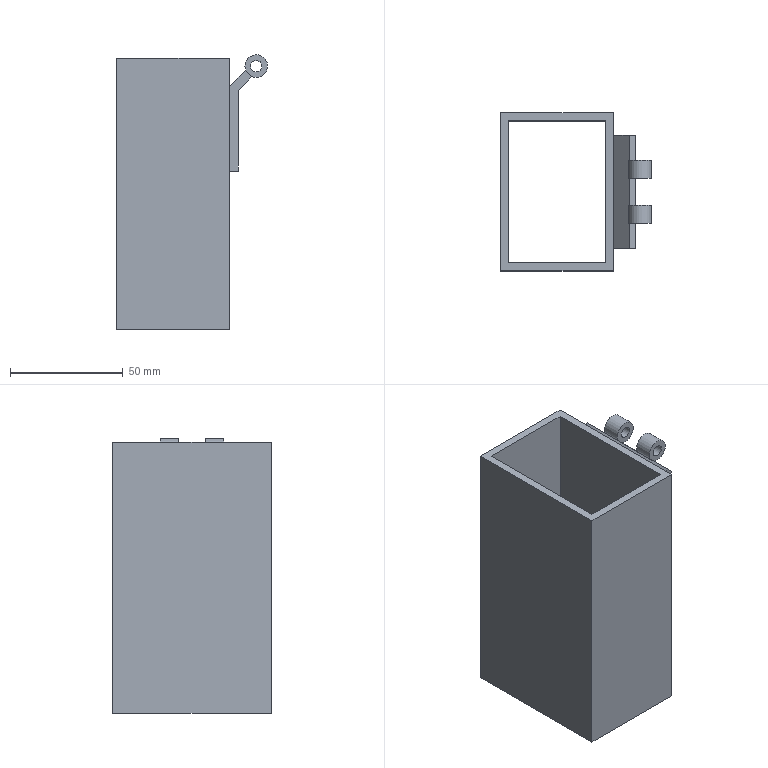Part | NX | features solid 2 | 1 solid | 25 faces | box 66.879 x 70 x 121.464 mm | volume 105008 mm3 | plane 21 | cylinder 4 | commonest cylinder face diameters 5 x2 10 x2
STEP:
#1=CARTESIAN_POINT('',(-1609.757,505.,4.586));
#2=VERTEX_POINT('',#1);
#3=CARTESIAN_POINT('',(-1609.757,455.,4.586));
#4=VERTEX_POINT('',#3);
#5=CARTESIAN_POINT('',(-1609.757,505.,4.586));
#6=DIRECTION('',(0.,1.,0.));
#7=VECTOR('',#6,1000.);
#8=LINE('',#5,#7);
#9=EDGE_CURVE('',#2,#4,#8,.F.);
#10=ORIENTED_EDGE('',*,*,#9,.T.);
#11=CARTESIAN_POINT('',(-1609.757,455.,-31.172));
#12=VERTEX_POINT('',#11);
#13=CARTESIAN_POINT('',(-1609.757,455.,18.828));
#14=DIRECTION('',(0.,0.,1.));
#15=VECTOR('',#14,1000.);
#16=LINE('',#13,#15);
#17=EDGE_CURVE('',#4,#12,#16,.F.);
#18=ORIENTED_EDGE('',*,*,#17,.T.);
#19=CARTESIAN_POINT('',(-1609.757,505.,-31.172));
#20=VERTEX_POINT('',#19);
#21=CARTESIAN_POINT('',(-1609.757,505.,-31.172));
#22=DIRECTION('',(0.,-1.,0.));
#23=VECTOR('',#22,1000.);
#24=LINE('',#21,#23);
#25=EDGE_CURVE('',#20,#12,#24,.T.);
#26=ORIENTED_EDGE('',*,*,#25,.F.);
#27=CARTESIAN_POINT('',(-1609.757,505.,18.828));
#28=DIRECTION('',(0.,0.,1.));
#29=VECTOR('',#28,1000.);
#30=LINE('',#27,#29);
#31=EDGE_CURVE('',#2,#20,#30,.F.);
#32=ORIENTED_EDGE('',*,*,#31,.F.);
#33=EDGE_LOOP('',(#10,#18,#26,#32));
#34=FACE_BOUND('',#33,.T.);
#35=CARTESIAN_POINT('',(-1609.757,505.,18.828));
#36=DIRECTION('',(1.,0.,0.));
#37=DIRECTION('',(0.,-1.,0.));
#38=AXIS2_PLACEMENT_3D('',#35,#36,#37);
#39=PLANE('',#38);
#40=ADVANCED_FACE('',(#34),#39,.T.);
#41=CARTESIAN_POINT('',(-1606.687,455.,13.313));
#42=VERTEX_POINT('',#41);
#43=CARTESIAN_POINT('',(-1613.757,455.,6.243));
#44=VERTEX_POINT('',#43);
#45=CARTESIAN_POINT('',(-1605.464,455.,14.536));
#46=DIRECTION('',(0.7071,0.,0.7071));
#47=VECTOR('',#46,1000.);
#48=LINE('',#45,#47);
#49=EDGE_CURVE('',#42,#44,#48,.F.);
#50=ORIENTED_EDGE('',*,*,#49,.T.);
#51=CARTESIAN_POINT('',(-1613.757,455.,-31.172));
#52=VERTEX_POINT('',#51);
#53=CARTESIAN_POINT('',(-1613.757,455.,18.828));
#54=DIRECTION('',(0.,0.,1.));
#55=VECTOR('',#54,1000.);
#56=LINE('',#53,#55);
#57=EDGE_CURVE('',#44,#52,#56,.F.);
#58=ORIENTED_EDGE('',*,*,#57,.T.);
#59=CARTESIAN_POINT('',(-1609.757,455.,-31.172));
#60=DIRECTION('',(-1.,0.,0.));
#61=VECTOR('',#60,1000.);
#62=LINE('',#59,#61);
#63=EDGE_CURVE('',#12,#52,#62,.T.);
#64=ORIENTED_EDGE('',*,*,#63,.F.);
#65=ORIENTED_EDGE('',*,*,#17,.F.);
#66=CARTESIAN_POINT('',(-1603.859,455.,10.485));
#67=VERTEX_POINT('',#66);
#68=CARTESIAN_POINT('',(-1614.707,455.,-0.364));
#69=DIRECTION('',(-0.7071,0.,-0.7071));
#70=VECTOR('',#69,1000.);
#71=LINE('',#68,#70);
#72=EDGE_CURVE('',#4,#67,#71,.F.);
#73=ORIENTED_EDGE('',*,*,#72,.T.);
#74=CARTESIAN_POINT('',(-1608.808,455.,15.434));
#75=DIRECTION('',(-0.7071,0.,0.7071));
#76=VECTOR('',#75,1000.);
#77=LINE('',#74,#76);
#78=EDGE_CURVE('',#42,#67,#77,.F.);
#79=ORIENTED_EDGE('',*,*,#78,.F.);
#80=EDGE_LOOP('',(#50,#58,#64,#65,#73,#79));
#81=FACE_BOUND('',#80,.T.);
#82=CARTESIAN_POINT('',(-1609.757,455.,18.828));
#83=DIRECTION('',(0.,-1.,0.));
#84=DIRECTION('',(-1.,0.,0.));
#85=AXIS2_PLACEMENT_3D('',#82,#83,#84);
#86=PLANE('',#85);
#87=ADVANCED_FACE('',(#81),#86,.T.);
#88=CARTESIAN_POINT('',(-1606.687,505.,13.313));
#89=VERTEX_POINT('',#88);
#90=CARTESIAN_POINT('',(-1613.757,505.,6.243));
#91=VERTEX_POINT('',#90);
#92=CARTESIAN_POINT('',(-1617.536,505.,2.464));
#93=DIRECTION('',(-0.7071,0.,-0.7071));
#94=VECTOR('',#93,1000.);
#95=LINE('',#92,#94);
#96=EDGE_CURVE('',#89,#91,#95,.T.);
#97=ORIENTED_EDGE('',*,*,#96,.F.);
#98=CARTESIAN_POINT('',(-1603.859,505.,10.485));
#99=VERTEX_POINT('',#98);
#100=CARTESIAN_POINT('',(-1608.808,505.,15.434));
#101=DIRECTION('',(-0.7071,0.,0.7071));
#102=VECTOR('',#101,1000.);
#103=LINE('',#100,#102);
#104=EDGE_CURVE('',#99,#89,#103,.T.);
#105=ORIENTED_EDGE('',*,*,#104,.F.);
#106=CARTESIAN_POINT('',(-1614.707,505.,-0.364));
#107=DIRECTION('',(0.7071,0.,0.7071));
#108=VECTOR('',#107,1000.);
#109=LINE('',#106,#108);
#110=EDGE_CURVE('',#2,#99,#109,.T.);
#111=ORIENTED_EDGE('',*,*,#110,.F.);
#112=ORIENTED_EDGE('',*,*,#31,.T.);
#113=CARTESIAN_POINT('',(-1613.757,505.,-31.172));
#114=VERTEX_POINT('',#113);
#115=CARTESIAN_POINT('',(-1609.757,505.,-31.172));
#116=DIRECTION('',(-1.,0.,0.));
#117=VECTOR('',#116,1000.);
#118=LINE('',#115,#117);
#119=EDGE_CURVE('',#20,#114,#118,.T.);
#120=ORIENTED_EDGE('',*,*,#119,.T.);
#121=CARTESIAN_POINT('',(-1613.757,505.,18.828));
#122=DIRECTION('',(0.,0.,1.));
#123=VECTOR('',#122,1000.);
#124=LINE('',#121,#123);
#125=EDGE_CURVE('',#91,#114,#124,.F.);
#126=ORIENTED_EDGE('',*,*,#125,.F.);
#127=EDGE_LOOP('',(#97,#105,#111,#112,#120,#126));
#128=FACE_BOUND('',#127,.T.);
#129=CARTESIAN_POINT('',(-1609.757,505.,18.828));
#130=DIRECTION('',(0.,-1.,0.));
#131=DIRECTION('',(-1.,0.,0.));
#132=AXIS2_PLACEMENT_3D('',#129,#130,#131);
#133=PLANE('',#132);
#134=ADVANCED_FACE('',(#128),#133,.F.);
#135=CARTESIAN_POINT('',(-1613.757,505.,-31.172));
#136=DIRECTION('',(0.,-1.,0.));
#137=VECTOR('',#136,1000.);
#138=LINE('',#135,#137);
#139=EDGE_CURVE('',#114,#52,#138,.T.);
#140=ORIENTED_EDGE('',*,*,#139,.F.);
#141=ORIENTED_EDGE('',*,*,#119,.F.);
#142=ORIENTED_EDGE('',*,*,#25,.T.);
#143=ORIENTED_EDGE('',*,*,#63,.T.);
#144=EDGE_LOOP('',(#140,#141,#142,#143));
#145=FACE_BOUND('',#144,.T.);
#146=CARTESIAN_POINT('',(-1609.757,505.,-31.172));
#147=DIRECTION('',(0.,0.,1.));
#148=DIRECTION('',(0.,-1.,0.));
#149=AXIS2_PLACEMENT_3D('',#146,#147,#148);
#150=PLANE('',#149);
#151=ADVANCED_FACE('',(#145),#150,.F.);
#152=CARTESIAN_POINT('',(-1613.757,505.,6.243));
#153=DIRECTION('',(0.,-1.,0.));
#154=VECTOR('',#153,1000.);
#155=LINE('',#152,#154);
#156=EDGE_CURVE('',#91,#44,#155,.T.);
#157=ORIENTED_EDGE('',*,*,#156,.T.);
#158=ORIENTED_EDGE('',*,*,#49,.F.);
#159=CARTESIAN_POINT('',(-1606.687,505.,13.313));
#160=DIRECTION('',(0.,1.,0.));
#161=VECTOR('',#160,1000.);
#162=LINE('',#159,#161);
#163=EDGE_CURVE('',#89,#42,#162,.F.);
#164=ORIENTED_EDGE('',*,*,#163,.F.);
#165=ORIENTED_EDGE('',*,*,#96,.T.);
#166=EDGE_LOOP('',(#157,#158,#164,#165));
#167=FACE_BOUND('',#166,.T.);
#168=CARTESIAN_POINT('',(-1617.536,505.,2.464));
#169=DIRECTION('',(-0.7071,0.,0.7071));
#170=DIRECTION('',(0.,-1.,0.));
#171=AXIS2_PLACEMENT_3D('',#168,#169,#170);
#172=PLANE('',#171);
#173=ADVANCED_FACE('',(#167),#172,.T.);
#174=ORIENTED_EDGE('',*,*,#72,.F.);
#175=ORIENTED_EDGE('',*,*,#9,.F.);
#176=ORIENTED_EDGE('',*,*,#110,.T.);
#177=CARTESIAN_POINT('',(-1603.859,505.,10.485));
#178=DIRECTION('',(0.,1.,0.));
#179=VECTOR('',#178,1000.);
#180=LINE('',#177,#179);
#181=EDGE_CURVE('',#67,#99,#180,.T.);
#182=ORIENTED_EDGE('',*,*,#181,.F.);
#183=EDGE_LOOP('',(#174,#175,#176,#182));
#184=FACE_BOUND('',#183,.T.);
#185=CARTESIAN_POINT('',(-1614.707,505.,-0.364));
#186=DIRECTION('',(-0.7071,0.,0.7071));
#187=DIRECTION('',(0.,-1.,0.));
#188=AXIS2_PLACEMENT_3D('',#185,#186,#187);
#189=PLANE('',#188);
#190=ADVANCED_FACE('',(#184),#189,.F.);
#191=CARTESIAN_POINT('',(-1606.263,466.,12.889));
#192=VERTEX_POINT('',#191);
#193=CARTESIAN_POINT('',(-1606.263,474.,12.889));
#194=VERTEX_POINT('',#193);
#195=CARTESIAN_POINT('',(-1606.263,455.,12.889));
#196=DIRECTION('',(0.,1.,0.));
#197=VECTOR('',#196,1000.);
#198=LINE('',#195,#197);
#199=EDGE_CURVE('',#192,#194,#198,.T.);
#200=ORIENTED_EDGE('',*,*,#199,.T.);
#201=CARTESIAN_POINT('',(-1604.283,474.,10.909));
#202=VERTEX_POINT('',#201);
#203=CARTESIAN_POINT('',(-1608.808,474.,15.434));
#204=DIRECTION('',(0.7071,0.,-0.7071));
#205=VECTOR('',#204,1000.);
#206=LINE('',#203,#205);
#207=EDGE_CURVE('',#194,#202,#206,.T.);
#208=ORIENTED_EDGE('',*,*,#207,.T.);
#209=CARTESIAN_POINT('',(-1604.283,466.,10.909));
#210=VERTEX_POINT('',#209);
#211=CARTESIAN_POINT('',(-1604.283,455.,10.909));
#212=DIRECTION('',(0.,1.,0.));
#213=VECTOR('',#212,1000.);
#214=LINE('',#211,#213);
#215=EDGE_CURVE('',#202,#210,#214,.F.);
#216=ORIENTED_EDGE('',*,*,#215,.T.);
#217=CARTESIAN_POINT('',(-1608.808,466.,15.434));
#218=DIRECTION('',(0.7071,0.,-0.7071));
#219=VECTOR('',#218,1000.);
#220=LINE('',#217,#219);
#221=EDGE_CURVE('',#192,#210,#220,.T.);
#222=ORIENTED_EDGE('',*,*,#221,.F.);
#223=EDGE_LOOP('',(#200,#208,#216,#222));
#224=FACE_BOUND('',#223,.T.);
#225=CARTESIAN_POINT('',(-1606.263,486.,12.889));
#226=VERTEX_POINT('',#225);
#227=CARTESIAN_POINT('',(-1606.263,494.,12.889));
#228=VERTEX_POINT('',#227);
#229=CARTESIAN_POINT('',(-1606.263,475.,12.889));
#230=DIRECTION('',(0.,1.,0.));
#231=VECTOR('',#230,1000.);
#232=LINE('',#229,#231);
#233=EDGE_CURVE('',#226,#228,#232,.T.);
#234=ORIENTED_EDGE('',*,*,#233,.T.);
#235=CARTESIAN_POINT('',(-1604.283,494.,10.909));
#236=VERTEX_POINT('',#235);
#237=CARTESIAN_POINT('',(-1608.808,494.,15.434));
#238=DIRECTION('',(0.7071,0.,-0.7071));
#239=VECTOR('',#238,1000.);
#240=LINE('',#237,#239);
#241=EDGE_CURVE('',#228,#236,#240,.T.);
#242=ORIENTED_EDGE('',*,*,#241,.T.);
#243=CARTESIAN_POINT('',(-1604.283,486.,10.909));
#244=VERTEX_POINT('',#243);
#245=CARTESIAN_POINT('',(-1604.283,475.,10.909));
#246=DIRECTION('',(0.,1.,0.));
#247=VECTOR('',#246,1000.);
#248=LINE('',#245,#247);
#249=EDGE_CURVE('',#236,#244,#248,.F.);
#250=ORIENTED_EDGE('',*,*,#249,.T.);
#251=CARTESIAN_POINT('',(-1608.808,486.,15.434));
#252=DIRECTION('',(0.7071,0.,-0.7071));
#253=VECTOR('',#252,1000.);
#254=LINE('',#251,#253);
#255=EDGE_CURVE('',#226,#244,#254,.T.);
#256=ORIENTED_EDGE('',*,*,#255,.F.);
#257=EDGE_LOOP('',(#234,#242,#250,#256));
#258=FACE_BOUND('',#257,.T.);
#259=ORIENTED_EDGE('',*,*,#163,.T.);
#260=ORIENTED_EDGE('',*,*,#78,.T.);
#261=ORIENTED_EDGE('',*,*,#181,.T.);
#262=ORIENTED_EDGE('',*,*,#104,.T.);
#263=EDGE_LOOP('',(#259,#260,#261,#262));
#264=FACE_BOUND('',#263,.T.);
#265=CARTESIAN_POINT('',(-1608.808,505.,15.434));
#266=DIRECTION('',(-0.7071,0.,-0.7071));
#267=DIRECTION('',(0.7071,0.,-0.7071));
#268=AXIS2_PLACEMENT_3D('',#265,#266,#267);
#269=PLANE('',#268);
#270=ADVANCED_FACE('',(#224,#258,#264),#269,.F.);
#271=CARTESIAN_POINT('',(-1613.757,515.,-101.172));
#272=VERTEX_POINT('',#271);
#273=CARTESIAN_POINT('',(-1613.757,445.,-101.172));
#274=VERTEX_POINT('',#273);
#275=CARTESIAN_POINT('',(-1613.757,530.,-101.172));
#276=DIRECTION('',(0.,1.,0.));
#277=VECTOR('',#276,1000.);
#278=LINE('',#275,#277);
#279=EDGE_CURVE('',#272,#274,#278,.F.);
#280=ORIENTED_EDGE('',*,*,#279,.F.);
#281=CARTESIAN_POINT('',(-1613.757,515.,18.828));
#282=VERTEX_POINT('',#281);
#283=CARTESIAN_POINT('',(-1613.757,515.,18.828));
#284=DIRECTION('',(0.,0.,1.));
#285=VECTOR('',#284,1000.);
#286=LINE('',#283,#285);
#287=EDGE_CURVE('',#282,#272,#286,.F.);
#288=ORIENTED_EDGE('',*,*,#287,.F.);
#289=CARTESIAN_POINT('',(-1613.757,445.,18.828));
#290=VERTEX_POINT('',#289);
#291=CARTESIAN_POINT('',(-1613.757,530.,18.828));
#292=DIRECTION('',(0.,-1.,0.));
#293=VECTOR('',#292,1000.);
#294=LINE('',#291,#293);
#295=EDGE_CURVE('',#282,#290,#294,.T.);
#296=ORIENTED_EDGE('',*,*,#295,.T.);
#297=CARTESIAN_POINT('',(-1613.757,445.,18.828));
#298=DIRECTION('',(0.,0.,-1.));
#299=VECTOR('',#298,1000.);
#300=LINE('',#297,#299);
#301=EDGE_CURVE('',#290,#274,#300,.T.);
#302=ORIENTED_EDGE('',*,*,#301,.T.);
#303=EDGE_LOOP('',(#280,#288,#296,#302));
#304=FACE_BOUND('',#303,.T.);
#305=ORIENTED_EDGE('',*,*,#57,.F.);
#306=ORIENTED_EDGE('',*,*,#156,.F.);
#307=ORIENTED_EDGE('',*,*,#125,.T.);
#308=ORIENTED_EDGE('',*,*,#139,.T.);
#309=EDGE_LOOP('',(#305,#306,#307,#308));
#310=FACE_BOUND('',#309,.T.);
#311=CARTESIAN_POINT('',(-1613.757,530.,18.828));
#312=DIRECTION('',(1.,0.,0.));
#313=DIRECTION('',(0.,-1.,0.));
#314=AXIS2_PLACEMENT_3D('',#311,#312,#313);
#315=PLANE('',#314);
#316=ADVANCED_FACE('',(#304,#310),#315,.T.);
#317=ORIENTED_EDGE('',*,*,#301,.F.);
#318=CARTESIAN_POINT('',(-1663.757,445.,18.828));
#319=VERTEX_POINT('',#318);
#320=CARTESIAN_POINT('',(-1613.757,445.,18.828));
#321=DIRECTION('',(1.,0.,0.));
#322=VECTOR('',#321,1000.);
#323=LINE('',#320,#322);
#324=EDGE_CURVE('',#290,#319,#323,.F.);
#325=ORIENTED_EDGE('',*,*,#324,.T.);
#326=CARTESIAN_POINT('',(-1663.757,445.,-101.172));
#327=VERTEX_POINT('',#326);
#328=CARTESIAN_POINT('',(-1663.757,445.,18.828));
#329=DIRECTION('',(0.,0.,1.));
#330=VECTOR('',#329,1000.);
#331=LINE('',#328,#330);
#332=EDGE_CURVE('',#319,#327,#331,.F.);
#333=ORIENTED_EDGE('',*,*,#332,.T.);
#334=CARTESIAN_POINT('',(-1613.757,445.,-101.172));
#335=DIRECTION('',(1.,0.,0.));
#336=VECTOR('',#335,1000.);
#337=LINE('',#334,#336);
#338=EDGE_CURVE('',#274,#327,#337,.F.);
#339=ORIENTED_EDGE('',*,*,#338,.F.);
#340=EDGE_LOOP('',(#317,#325,#333,#339));
#341=FACE_BOUND('',#340,.T.);
#342=CARTESIAN_POINT('',(-1613.757,445.,18.828));
#343=DIRECTION('',(0.,-1.,0.));
#344=DIRECTION('',(-1.,0.,0.));
#345=AXIS2_PLACEMENT_3D('',#342,#343,#344);
#346=PLANE('',#345);
#347=ADVANCED_FACE('',(#341),#346,.T.);
#348=CARTESIAN_POINT('',(-1617.257,511.5,18.828));
#349=VERTEX_POINT('',#348);
#350=CARTESIAN_POINT('',(-1617.257,448.5,18.828));
#351=VERTEX_POINT('',#350);
#352=CARTESIAN_POINT('',(-1617.257,530.,18.828));
#353=DIRECTION('',(0.,-1.,0.));
#354=VECTOR('',#353,1000.);
#355=LINE('',#352,#354);
#356=EDGE_CURVE('',#349,#351,#355,.T.);
#357=ORIENTED_EDGE('',*,*,#356,.F.);
#358=CARTESIAN_POINT('',(-1617.257,511.5,-101.172));
#359=VERTEX_POINT('',#358);
#360=CARTESIAN_POINT('',(-1617.257,511.5,18.828));
#361=DIRECTION('',(0.,0.,1.));
#362=VECTOR('',#361,1000.);
#363=LINE('',#360,#362);
#364=EDGE_CURVE('',#359,#349,#363,.T.);
#365=ORIENTED_EDGE('',*,*,#364,.F.);
#366=CARTESIAN_POINT('',(-1617.257,448.5,-101.172));
#367=VERTEX_POINT('',#366);
#368=CARTESIAN_POINT('',(-1617.257,530.,-101.172));
#369=DIRECTION('',(0.,-1.,0.));
#370=VECTOR('',#369,1000.);
#371=LINE('',#368,#370);
#372=EDGE_CURVE('',#359,#367,#371,.T.);
#373=ORIENTED_EDGE('',*,*,#372,.T.);
#374=CARTESIAN_POINT('',(-1617.257,448.5,18.828));
#375=DIRECTION('',(0.,0.,-1.));
#376=VECTOR('',#375,1000.);
#377=LINE('',#374,#376);
#378=EDGE_CURVE('',#351,#367,#377,.T.);
#379=ORIENTED_EDGE('',*,*,#378,.F.);
#380=EDGE_LOOP('',(#357,#365,#373,#379));
#381=FACE_BOUND('',#380,.T.);
#382=CARTESIAN_POINT('',(-1617.257,530.,18.828));
#383=DIRECTION('',(1.,0.,0.));
#384=DIRECTION('',(0.,-1.,0.));
#385=AXIS2_PLACEMENT_3D('',#382,#383,#384);
#386=PLANE('',#385);
#387=ADVANCED_FACE('',(#381),#386,.F.);
#388=CARTESIAN_POINT('',(-1663.757,515.,18.828));
#389=VERTEX_POINT('',#388);
#390=CARTESIAN_POINT('',(-1613.757,515.,18.828));
#391=DIRECTION('',(-1.,0.,0.));
#392=VECTOR('',#391,1000.);
#393=LINE('',#390,#392);
#394=EDGE_CURVE('',#282,#389,#393,.T.);
#395=ORIENTED_EDGE('',*,*,#394,.F.);
#396=ORIENTED_EDGE('',*,*,#287,.T.);
#397=CARTESIAN_POINT('',(-1663.757,515.,-101.172));
#398=VERTEX_POINT('',#397);
#399=CARTESIAN_POINT('',(-1613.757,515.,-101.172));
#400=DIRECTION('',(-1.,0.,0.));
#401=VECTOR('',#400,1000.);
#402=LINE('',#399,#401);
#403=EDGE_CURVE('',#272,#398,#402,.T.);
#404=ORIENTED_EDGE('',*,*,#403,.T.);
#405=CARTESIAN_POINT('',(-1663.757,515.,18.828));
#406=DIRECTION('',(0.,0.,-1.));
#407=VECTOR('',#406,1000.);
#408=LINE('',#405,#407);
#409=EDGE_CURVE('',#389,#398,#408,.T.);
#410=ORIENTED_EDGE('',*,*,#409,.F.);
#411=EDGE_LOOP('',(#395,#396,#404,#410));
#412=FACE_BOUND('',#411,.T.);
#413=CARTESIAN_POINT('',(-1613.757,515.,18.828));
#414=DIRECTION('',(0.,-1.,0.));
#415=DIRECTION('',(-1.,0.,0.));
#416=AXIS2_PLACEMENT_3D('',#413,#414,#415);
#417=PLANE('',#416);
#418=ADVANCED_FACE('',(#412),#417,.F.);
#419=CARTESIAN_POINT('',(-1660.257,511.5,-101.172));
#420=VERTEX_POINT('',#419);
#421=CARTESIAN_POINT('',(-1660.257,448.5,-101.172));
#422=VERTEX_POINT('',#421);
#423=CARTESIAN_POINT('',(-1660.257,530.,-101.172));
#424=DIRECTION('',(0.,-1.,0.));
#425=VECTOR('',#424,1000.);
#426=LINE('',#423,#425);
#427=EDGE_CURVE('',#420,#422,#426,.T.);
#428=ORIENTED_EDGE('',*,*,#427,.T.);
#429=CARTESIAN_POINT('',(-1613.757,448.5,-101.172));
#430=DIRECTION('',(-1.,0.,0.));
#431=VECTOR('',#430,1000.);
#432=LINE('',#429,#431);
#433=EDGE_CURVE('',#367,#422,#432,.T.);
#434=ORIENTED_EDGE('',*,*,#433,.F.);
#435=ORIENTED_EDGE('',*,*,#372,.F.);
#436=CARTESIAN_POINT('',(-1613.757,511.5,-101.172));
#437=DIRECTION('',(-1.,0.,0.));
#438=VECTOR('',#437,1000.);
#439=LINE('',#436,#438);
#440=EDGE_CURVE('',#359,#420,#439,.T.);
#441=ORIENTED_EDGE('',*,*,#440,.T.);
#442=EDGE_LOOP('',(#428,#434,#435,#441));
#443=FACE_BOUND('',#442,.T.);
#444=ORIENTED_EDGE('',*,*,#403,.F.);
#445=ORIENTED_EDGE('',*,*,#279,.T.);
#446=ORIENTED_EDGE('',*,*,#338,.T.);
#447=CARTESIAN_POINT('',(-1663.757,522.,-101.172));
#448=DIRECTION('',(0.,1.,0.));
#449=VECTOR('',#448,1000.);
#450=LINE('',#447,#449);
#451=EDGE_CURVE('',#327,#398,#450,.T.);
#452=ORIENTED_EDGE('',*,*,#451,.T.);
#453=EDGE_LOOP('',(#444,#445,#446,#452));
#454=FACE_BOUND('',#453,.T.);
#455=CARTESIAN_POINT('',(-1613.757,530.,-101.172));
#456=DIRECTION('',(0.,0.,1.));
#457=DIRECTION('',(0.,-1.,0.));
#458=AXIS2_PLACEMENT_3D('',#455,#456,#457);
#459=PLANE('',#458);
#460=ADVANCED_FACE('',(#443,#454),#459,.F.);
#461=CARTESIAN_POINT('',(-1660.257,511.5,18.828));
#462=VERTEX_POINT('',#461);
#463=CARTESIAN_POINT('',(-1613.757,511.5,18.828));
#464=DIRECTION('',(-1.,0.,0.));
#465=VECTOR('',#464,1000.);
#466=LINE('',#463,#465);
#467=EDGE_CURVE('',#349,#462,#466,.T.);
#468=ORIENTED_EDGE('',*,*,#467,.F.);
#469=ORIENTED_EDGE('',*,*,#356,.T.);
#470=CARTESIAN_POINT('',(-1660.257,448.5,18.828));
#471=VERTEX_POINT('',#470);
#472=CARTESIAN_POINT('',(-1613.757,448.5,18.828));
#473=DIRECTION('',(-1.,0.,0.));
#474=VECTOR('',#473,1000.);
#475=LINE('',#472,#474);
#476=EDGE_CURVE('',#351,#471,#475,.T.);
#477=ORIENTED_EDGE('',*,*,#476,.T.);
#478=CARTESIAN_POINT('',(-1660.257,530.,18.828));
#479=DIRECTION('',(0.,-1.,0.));
#480=VECTOR('',#479,1000.);
#481=LINE('',#478,#480);
#482=EDGE_CURVE('',#462,#471,#481,.T.);
#483=ORIENTED_EDGE('',*,*,#482,.F.);
#484=EDGE_LOOP('',(#468,#469,#477,#483));
#485=FACE_BOUND('',#484,.T.);
#486=CARTESIAN_POINT('',(-1663.757,530.,18.828));
#487=DIRECTION('',(0.,1.,0.));
#488=VECTOR('',#487,1000.);
#489=LINE('',#486,#488);
#490=EDGE_CURVE('',#319,#389,#489,.T.);
#491=ORIENTED_EDGE('',*,*,#490,.F.);
#492=ORIENTED_EDGE('',*,*,#324,.F.);
#493=ORIENTED_EDGE('',*,*,#295,.F.);
#494=ORIENTED_EDGE('',*,*,#394,.T.);
#495=EDGE_LOOP('',(#491,#492,#493,#494));
#496=FACE_BOUND('',#495,.T.);
#497=CARTESIAN_POINT('',(-1613.757,530.,18.828));
#498=DIRECTION('',(0.,0.,1.));
#499=DIRECTION('',(0.,-1.,0.));
#500=AXIS2_PLACEMENT_3D('',#497,#498,#499);
#501=PLANE('',#500);
#502=ADVANCED_FACE('',(#485,#496),#501,.T.);
#503=CARTESIAN_POINT('',(-1660.257,511.5,18.828));
#504=DIRECTION('',(0.,0.,-1.));
#505=VECTOR('',#504,1000.);
#506=LINE('',#503,#505);
#507=EDGE_CURVE('',#462,#420,#506,.T.);
#508=ORIENTED_EDGE('',*,*,#507,.T.);
#509=ORIENTED_EDGE('',*,*,#440,.F.);
#510=ORIENTED_EDGE('',*,*,#364,.T.);
#511=ORIENTED_EDGE('',*,*,#467,.T.);
#512=EDGE_LOOP('',(#508,#509,#510,#511));
#513=FACE_BOUND('',#512,.T.);
#514=CARTESIAN_POINT('',(-1613.757,511.5,18.828));
#515=DIRECTION('',(0.,-1.,0.));
#516=DIRECTION('',(0.,0.,-1.));
#517=AXIS2_PLACEMENT_3D('',#514,#515,#516);
#518=PLANE('',#517);
#519=ADVANCED_FACE('',(#513),#518,.T.);
#520=ORIENTED_EDGE('',*,*,#409,.T.);
#521=ORIENTED_EDGE('',*,*,#451,.F.);
#522=ORIENTED_EDGE('',*,*,#332,.F.);
#523=ORIENTED_EDGE('',*,*,#490,.T.);
#524=EDGE_LOOP('',(#520,#521,#522,#523));
#525=FACE_BOUND('',#524,.T.);
#526=CARTESIAN_POINT('',(-1663.757,522.,18.828));
#527=DIRECTION('',(-1.,0.,0.));
#528=DIRECTION('',(0.,0.,-1.));
#529=AXIS2_PLACEMENT_3D('',#526,#527,#528);
#530=PLANE('',#529);
#531=ADVANCED_FACE('',(#525),#530,.T.);
#532=CARTESIAN_POINT('',(-1660.257,448.5,18.828));
#533=DIRECTION('',(0.,0.,-1.));
#534=VECTOR('',#533,1000.);
#535=LINE('',#532,#534);
#536=EDGE_CURVE('',#471,#422,#535,.T.);
#537=ORIENTED_EDGE('',*,*,#536,.F.);
#538=ORIENTED_EDGE('',*,*,#476,.F.);
#539=ORIENTED_EDGE('',*,*,#378,.T.);
#540=ORIENTED_EDGE('',*,*,#433,.T.);
#541=EDGE_LOOP('',(#537,#538,#539,#540));
#542=FACE_BOUND('',#541,.T.);
#543=CARTESIAN_POINT('',(-1613.757,448.5,18.828));
#544=DIRECTION('',(0.,1.,0.));
#545=DIRECTION('',(0.,0.,-1.));
#546=AXIS2_PLACEMENT_3D('',#543,#544,#545);
#547=PLANE('',#546);
#548=ADVANCED_FACE('',(#542),#547,.T.);
#549=ORIENTED_EDGE('',*,*,#482,.T.);
#550=ORIENTED_EDGE('',*,*,#536,.T.);
#551=ORIENTED_EDGE('',*,*,#427,.F.);
#552=ORIENTED_EDGE('',*,*,#507,.F.);
#553=EDGE_LOOP('',(#549,#550,#551,#552));
#554=FACE_BOUND('',#553,.T.);
#555=CARTESIAN_POINT('',(-1660.257,530.,18.828));
#556=DIRECTION('',(1.,0.,0.));
#557=DIRECTION('',(0.,0.,1.));
#558=AXIS2_PLACEMENT_3D('',#555,#556,#557);
#559=PLANE('',#558);
#560=ADVANCED_FACE('',(#554),#559,.T.);
#561=CARTESIAN_POINT('',(-1601.879,494.,15.293));
#562=DIRECTION('',(0.,1.,0.));
#563=DIRECTION('',(0.,0.,-1.));
#564=AXIS2_PLACEMENT_3D('',#561,#562,#563);
#565=CIRCLE('',#564,5.);
#566=EDGE_CURVE('',#228,#236,#565,.T.);
#567=ORIENTED_EDGE('',*,*,#566,.F.);
#568=ORIENTED_EDGE('',*,*,#233,.F.);
#569=CARTESIAN_POINT('',(-1601.879,486.,15.293));
#570=DIRECTION('',(0.,1.,0.));
#571=DIRECTION('',(0.,0.,-1.));
#572=AXIS2_PLACEMENT_3D('',#569,#570,#571);
#573=CIRCLE('',#572,5.);
#574=EDGE_CURVE('',#226,#244,#573,.T.);
#575=ORIENTED_EDGE('',*,*,#574,.T.);
#576=ORIENTED_EDGE('',*,*,#249,.F.);
#577=EDGE_LOOP('',(#567,#568,#575,#576));
#578=FACE_BOUND('',#577,.T.);
#579=CARTESIAN_POINT('',(-1601.879,475.,15.293));
#580=DIRECTION('',(0.,1.,0.));
#581=DIRECTION('',(0.,0.,1.));
#582=AXIS2_PLACEMENT_3D('',#579,#580,#581);
#583=CYLINDRICAL_SURFACE('',#582,5.);
#584=ADVANCED_FACE('',(#578),#583,.T.);
#585=CARTESIAN_POINT('',(-1601.879,486.,12.793));
#586=VERTEX_POINT('',#585);
#587=CARTESIAN_POINT('',(-1601.879,486.,15.293));
#588=DIRECTION('',(0.,1.,0.));
#589=DIRECTION('',(0.,0.,-1.));
#590=AXIS2_PLACEMENT_3D('',#587,#588,#589);
#591=CIRCLE('',#590,2.5);
#592=EDGE_CURVE('',#586,#586,#591,.T.);
#593=ORIENTED_EDGE('',*,*,#592,.T.);
#594=EDGE_LOOP('',(#593));
#595=FACE_BOUND('',#594,.T.);
#596=ORIENTED_EDGE('',*,*,#255,.T.);
#597=ORIENTED_EDGE('',*,*,#574,.F.);
#598=EDGE_LOOP('',(#596,#597));
#599=FACE_BOUND('',#598,.T.);
#600=CARTESIAN_POINT('',(-1601.879,486.,15.293));
#601=DIRECTION('',(0.,-1.,0.));
#602=DIRECTION('',(0.,0.,-1.));
#603=AXIS2_PLACEMENT_3D('',#600,#601,#602);
#604=PLANE('',#603);
#605=ADVANCED_FACE('',(#595,#599),#604,.T.);
#606=CARTESIAN_POINT('',(-1601.879,494.,12.793));
#607=VERTEX_POINT('',#606);
#608=CARTESIAN_POINT('',(-1601.879,494.,15.293));
#609=DIRECTION('',(0.,1.,0.));
#610=DIRECTION('',(0.,0.,-1.));
#611=AXIS2_PLACEMENT_3D('',#608,#609,#610);
#612=CIRCLE('',#611,2.5);
#613=EDGE_CURVE('',#607,#607,#612,.T.);
#614=ORIENTED_EDGE('',*,*,#613,.F.);
#615=EDGE_LOOP('',(#614));
#616=FACE_BOUND('',#615,.T.);
#617=ORIENTED_EDGE('',*,*,#566,.T.);
#618=ORIENTED_EDGE('',*,*,#241,.F.);
#619=EDGE_LOOP('',(#617,#618));
#620=FACE_BOUND('',#619,.T.);
#621=CARTESIAN_POINT('',(-1601.879,494.,15.293));
#622=DIRECTION('',(0.,-1.,0.));
#623=DIRECTION('',(0.,0.,-1.));
#624=AXIS2_PLACEMENT_3D('',#621,#622,#623);
#625=PLANE('',#624);
#626=ADVANCED_FACE('',(#616,#620),#625,.F.);
#627=ORIENTED_EDGE('',*,*,#592,.F.);
#628=EDGE_LOOP('',(#627));
#629=FACE_BOUND('',#628,.T.);
#630=ORIENTED_EDGE('',*,*,#613,.T.);
#631=EDGE_LOOP('',(#630));
#632=FACE_BOUND('',#631,.T.);
#633=CARTESIAN_POINT('',(-1601.879,495.,15.293));
#634=DIRECTION('',(0.,-1.,0.));
#635=DIRECTION('',(0.,0.,-1.));
#636=AXIS2_PLACEMENT_3D('',#633,#634,#635);
#637=CYLINDRICAL_SURFACE('',#636,2.5);
#638=ADVANCED_FACE('',(#629,#632),#637,.F.);
#639=CARTESIAN_POINT('',(-1601.879,474.,15.293));
#640=DIRECTION('',(0.,1.,0.));
#641=DIRECTION('',(0.,0.,-1.));
#642=AXIS2_PLACEMENT_3D('',#639,#640,#641);
#643=CIRCLE('',#642,5.);
#644=EDGE_CURVE('',#194,#202,#643,.T.);
#645=ORIENTED_EDGE('',*,*,#644,.F.);
#646=ORIENTED_EDGE('',*,*,#199,.F.);
#647=CARTESIAN_POINT('',(-1601.879,466.,15.293));
#648=DIRECTION('',(0.,1.,0.));
#649=DIRECTION('',(0.,0.,-1.));
#650=AXIS2_PLACEMENT_3D('',#647,#648,#649);
#651=CIRCLE('',#650,5.);
#652=EDGE_CURVE('',#192,#210,#651,.T.);
#653=ORIENTED_EDGE('',*,*,#652,.T.);
#654=ORIENTED_EDGE('',*,*,#215,.F.);
#655=EDGE_LOOP('',(#645,#646,#653,#654));
#656=FACE_BOUND('',#655,.T.);
#657=CARTESIAN_POINT('',(-1601.879,455.,15.293));
#658=DIRECTION('',(0.,1.,0.));
#659=DIRECTION('',(0.,0.,1.));
#660=AXIS2_PLACEMENT_3D('',#657,#658,#659);
#661=CYLINDRICAL_SURFACE('',#660,5.);
#662=ADVANCED_FACE('',(#656),#661,.T.);
#663=CARTESIAN_POINT('',(-1601.879,466.,12.793));
#664=VERTEX_POINT('',#663);
#665=CARTESIAN_POINT('',(-1601.879,466.,15.293));
#666=DIRECTION('',(0.,1.,0.));
#667=DIRECTION('',(0.,0.,-1.));
#668=AXIS2_PLACEMENT_3D('',#665,#666,#667);
#669=CIRCLE('',#668,2.5);
#670=EDGE_CURVE('',#664,#664,#669,.T.);
#671=ORIENTED_EDGE('',*,*,#670,.T.);
#672=EDGE_LOOP('',(#671));
#673=FACE_BOUND('',#672,.T.);
#674=ORIENTED_EDGE('',*,*,#221,.T.);
#675=ORIENTED_EDGE('',*,*,#652,.F.);
#676=EDGE_LOOP('',(#674,#675));
#677=FACE_BOUND('',#676,.T.);
#678=CARTESIAN_POINT('',(-1601.879,466.,15.293));
#679=DIRECTION('',(0.,-1.,0.));
#680=DIRECTION('',(0.,0.,-1.));
#681=AXIS2_PLACEMENT_3D('',#678,#679,#680);
#682=PLANE('',#681);
#683=ADVANCED_FACE('',(#673,#677),#682,.T.);
#684=CARTESIAN_POINT('',(-1601.879,474.,12.793));
#685=VERTEX_POINT('',#684);
#686=CARTESIAN_POINT('',(-1601.879,474.,15.293));
#687=DIRECTION('',(0.,1.,0.));
#688=DIRECTION('',(0.,0.,-1.));
#689=AXIS2_PLACEMENT_3D('',#686,#687,#688);
#690=CIRCLE('',#689,2.5);
#691=EDGE_CURVE('',#685,#685,#690,.T.);
#692=ORIENTED_EDGE('',*,*,#691,.F.);
#693=EDGE_LOOP('',(#692));
#694=FACE_BOUND('',#693,.T.);
#695=ORIENTED_EDGE('',*,*,#644,.T.);
#696=ORIENTED_EDGE('',*,*,#207,.F.);
#697=EDGE_LOOP('',(#695,#696));
#698=FACE_BOUND('',#697,.T.);
#699=CARTESIAN_POINT('',(-1601.879,474.,15.293));
#700=DIRECTION('',(0.,-1.,0.));
#701=DIRECTION('',(0.,0.,-1.));
#702=AXIS2_PLACEMENT_3D('',#699,#700,#701);
#703=PLANE('',#702);
#704=ADVANCED_FACE('',(#694,#698),#703,.F.);
#705=ORIENTED_EDGE('',*,*,#670,.F.);
#706=EDGE_LOOP('',(#705));
#707=FACE_BOUND('',#706,.T.);
#708=ORIENTED_EDGE('',*,*,#691,.T.);
#709=EDGE_LOOP('',(#708));
#710=FACE_BOUND('',#709,.T.);
#711=CARTESIAN_POINT('',(-1601.879,475.,15.293));
#712=DIRECTION('',(0.,-1.,0.));
#713=DIRECTION('',(0.,0.,-1.));
#714=AXIS2_PLACEMENT_3D('',#711,#712,#713);
#715=CYLINDRICAL_SURFACE('',#714,2.5);
#716=ADVANCED_FACE('',(#707,#710),#715,.F.);
#717=CLOSED_SHELL('',(#40,#87,#134,#151,#173,#190,#270,#316,#347,#387,#418,#460,#502,#519,#531,#548,#560,#584,#605,#626,#638,#662,#683,#704,#716));
#718=MANIFOLD_SOLID_BREP('',#717);
#719=(LENGTH_UNIT()NAMED_UNIT(*)SI_UNIT(.MILLI.,.METRE.));
#720=UNCERTAINTY_MEASURE_WITH_UNIT(LENGTH_MEASURE(0.00001),#719,'','');
#721=(NAMED_UNIT(*)PLANE_ANGLE_UNIT()SI_UNIT($,.RADIAN.));
#722=(NAMED_UNIT(*)SI_UNIT($,.STERADIAN.)SOLID_ANGLE_UNIT());
#723=(GEOMETRIC_REPRESENTATION_CONTEXT(3)GLOBAL_UNCERTAINTY_ASSIGNED_CONTEXT((#720))GLOBAL_UNIT_ASSIGNED_CONTEXT((#719,#721,#722))REPRESENTATION_CONTEXT('',''));
#724=ADVANCED_BREP_SHAPE_REPRESENTATION('',(#718),#723);